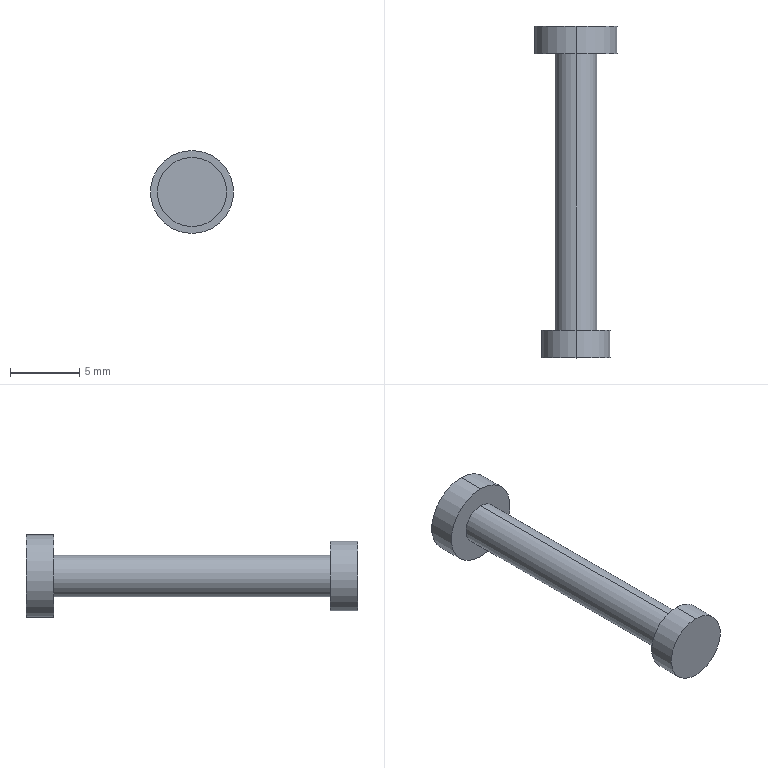Part | SolidWorks | features Revolution 1 | 1 solid | 10 faces | box 6 x 24 x 6 mm | volume 237.19 mm3 | cylinder 6 | plane 4 | commonest cylinder face diameters 3 x2 5 x2 6 x2
STEP:
#1=CARTESIAN_POINT('',(0.,22.,3.));
#2=VERTEX_POINT('',#1);
#3=CARTESIAN_POINT('',(0.,22.,-3.));
#4=VERTEX_POINT('',#3);
#5=CARTESIAN_POINT('',(0.,22.,0.));
#6=DIRECTION('',(0.,1.,0.));
#7=DIRECTION('',(0.,0.,1.));
#8=AXIS2_PLACEMENT_3D('',#5,#6,#7);
#9=CIRCLE('',#8,3.);
#10=EDGE_CURVE('',#2,#4,#9,.T.);
#11=ORIENTED_EDGE('',*,*,#10,.T.);
#12=CARTESIAN_POINT('',(0.,24.,-3.));
#13=VERTEX_POINT('',#12);
#14=CARTESIAN_POINT('',(0.,24.,-3.));
#15=DIRECTION('',(0.,1.,0.));
#16=VECTOR('',#15,1000.);
#17=LINE('',#14,#16);
#18=EDGE_CURVE('',#4,#13,#17,.T.);
#19=ORIENTED_EDGE('',*,*,#18,.T.);
#20=CARTESIAN_POINT('',(0.,24.,3.));
#21=VERTEX_POINT('',#20);
#22=CARTESIAN_POINT('',(0.,24.,0.));
#23=DIRECTION('',(0.,1.,0.));
#24=DIRECTION('',(0.,0.,1.));
#25=AXIS2_PLACEMENT_3D('',#22,#23,#24);
#26=CIRCLE('',#25,3.);
#27=EDGE_CURVE('',#21,#13,#26,.T.);
#28=ORIENTED_EDGE('',*,*,#27,.F.);
#29=CARTESIAN_POINT('',(0.,24.,3.));
#30=DIRECTION('',(0.,1.,0.));
#31=VECTOR('',#30,1000.);
#32=LINE('',#29,#31);
#33=EDGE_CURVE('',#2,#21,#32,.T.);
#34=ORIENTED_EDGE('',*,*,#33,.F.);
#35=EDGE_LOOP('',(#11,#19,#28,#34));
#36=FACE_OUTER_BOUND('',#35,.T.);
#37=CARTESIAN_POINT('',(0.,24.,0.));
#38=DIRECTION('',(0.,1.,0.));
#39=DIRECTION('',(0.,0.,1.));
#40=AXIS2_PLACEMENT_3D('',#37,#38,#39);
#41=CYLINDRICAL_SURFACE('',#40,3.);
#42=ADVANCED_FACE('',(#36),#41,.T.);
#43=CARTESIAN_POINT('',(0.,2.,1.5));
#44=VERTEX_POINT('',#43);
#45=CARTESIAN_POINT('',(0.,2.,-1.5));
#46=VERTEX_POINT('',#45);
#47=CARTESIAN_POINT('',(0.,2.,0.));
#48=DIRECTION('',(0.,1.,0.));
#49=DIRECTION('',(0.,0.,1.));
#50=AXIS2_PLACEMENT_3D('',#47,#48,#49);
#51=CIRCLE('',#50,1.5);
#52=EDGE_CURVE('',#44,#46,#51,.T.);
#53=ORIENTED_EDGE('',*,*,#52,.T.);
#54=CARTESIAN_POINT('',(0.,22.,-1.5));
#55=VERTEX_POINT('',#54);
#56=CARTESIAN_POINT('',(0.,24.,-1.5));
#57=DIRECTION('',(0.,1.,0.));
#58=VECTOR('',#57,1000.);
#59=LINE('',#56,#58);
#60=EDGE_CURVE('',#46,#55,#59,.T.);
#61=ORIENTED_EDGE('',*,*,#60,.T.);
#62=CARTESIAN_POINT('',(0.,22.,1.5));
#63=VERTEX_POINT('',#62);
#64=CARTESIAN_POINT('',(0.,22.,0.));
#65=DIRECTION('',(0.,1.,0.));
#66=DIRECTION('',(0.,0.,1.));
#67=AXIS2_PLACEMENT_3D('',#64,#65,#66);
#68=CIRCLE('',#67,1.5);
#69=EDGE_CURVE('',#63,#55,#68,.T.);
#70=ORIENTED_EDGE('',*,*,#69,.F.);
#71=CARTESIAN_POINT('',(0.,24.,1.5));
#72=DIRECTION('',(0.,1.,0.));
#73=VECTOR('',#72,1000.);
#74=LINE('',#71,#73);
#75=EDGE_CURVE('',#44,#63,#74,.T.);
#76=ORIENTED_EDGE('',*,*,#75,.F.);
#77=EDGE_LOOP('',(#53,#61,#70,#76));
#78=FACE_OUTER_BOUND('',#77,.T.);
#79=CARTESIAN_POINT('',(0.,24.,0.));
#80=DIRECTION('',(0.,1.,0.));
#81=DIRECTION('',(0.,0.,1.));
#82=AXIS2_PLACEMENT_3D('',#79,#80,#81);
#83=CYLINDRICAL_SURFACE('',#82,1.5);
#84=ADVANCED_FACE('',(#78),#83,.T.);
#85=CARTESIAN_POINT('',(0.,0.,2.5));
#86=VERTEX_POINT('',#85);
#87=CARTESIAN_POINT('',(0.,0.,-2.5));
#88=VERTEX_POINT('',#87);
#89=CARTESIAN_POINT('',(0.,0.,0.));
#90=DIRECTION('',(0.,1.,0.));
#91=DIRECTION('',(0.,0.,1.));
#92=AXIS2_PLACEMENT_3D('',#89,#90,#91);
#93=CIRCLE('',#92,2.5);
#94=EDGE_CURVE('',#86,#88,#93,.T.);
#95=ORIENTED_EDGE('',*,*,#94,.T.);
#96=CARTESIAN_POINT('',(0.,2.,-2.5));
#97=VERTEX_POINT('',#96);
#98=CARTESIAN_POINT('',(0.,24.,-2.5));
#99=DIRECTION('',(0.,1.,0.));
#100=VECTOR('',#99,1000.);
#101=LINE('',#98,#100);
#102=EDGE_CURVE('',#88,#97,#101,.T.);
#103=ORIENTED_EDGE('',*,*,#102,.T.);
#104=CARTESIAN_POINT('',(0.,2.,2.5));
#105=VERTEX_POINT('',#104);
#106=CARTESIAN_POINT('',(0.,2.,0.));
#107=DIRECTION('',(0.,1.,0.));
#108=DIRECTION('',(0.,0.,1.));
#109=AXIS2_PLACEMENT_3D('',#106,#107,#108);
#110=CIRCLE('',#109,2.5);
#111=EDGE_CURVE('',#105,#97,#110,.T.);
#112=ORIENTED_EDGE('',*,*,#111,.F.);
#113=CARTESIAN_POINT('',(0.,24.,2.5));
#114=DIRECTION('',(0.,1.,0.));
#115=VECTOR('',#114,1000.);
#116=LINE('',#113,#115);
#117=EDGE_CURVE('',#86,#105,#116,.T.);
#118=ORIENTED_EDGE('',*,*,#117,.F.);
#119=EDGE_LOOP('',(#95,#103,#112,#118));
#120=FACE_OUTER_BOUND('',#119,.T.);
#121=CARTESIAN_POINT('',(0.,24.,0.));
#122=DIRECTION('',(0.,1.,0.));
#123=DIRECTION('',(0.,0.,1.));
#124=AXIS2_PLACEMENT_3D('',#121,#122,#123);
#125=CYLINDRICAL_SURFACE('',#124,2.5);
#126=ADVANCED_FACE('',(#120),#125,.T.);
#127=ORIENTED_EDGE('',*,*,#94,.F.);
#128=CARTESIAN_POINT('',(0.,0.,0.));
#129=DIRECTION('',(0.,1.,0.));
#130=DIRECTION('',(0.,0.,1.));
#131=AXIS2_PLACEMENT_3D('',#128,#129,#130);
#132=CIRCLE('',#131,2.5);
#133=EDGE_CURVE('',#88,#86,#132,.T.);
#134=ORIENTED_EDGE('',*,*,#133,.F.);
#135=EDGE_LOOP('',(#127,#134));
#136=FACE_OUTER_BOUND('',#135,.T.);
#137=CARTESIAN_POINT('',(0.,0.,0.));
#138=DIRECTION('',(0.,1.,0.));
#139=DIRECTION('',(0.,0.,1.));
#140=AXIS2_PLACEMENT_3D('',#137,#138,#139);
#141=PLANE('',#140);
#142=ADVANCED_FACE('',(#136),#141,.F.);
#143=ORIENTED_EDGE('',*,*,#102,.F.);
#144=ORIENTED_EDGE('',*,*,#133,.T.);
#145=ORIENTED_EDGE('',*,*,#117,.T.);
#146=CARTESIAN_POINT('',(0.,2.,0.));
#147=DIRECTION('',(0.,1.,0.));
#148=DIRECTION('',(0.,0.,1.));
#149=AXIS2_PLACEMENT_3D('',#146,#147,#148);
#150=CIRCLE('',#149,2.5);
#151=EDGE_CURVE('',#97,#105,#150,.T.);
#152=ORIENTED_EDGE('',*,*,#151,.F.);
#153=EDGE_LOOP('',(#143,#144,#145,#152));
#154=FACE_OUTER_BOUND('',#153,.T.);
#155=CARTESIAN_POINT('',(0.,24.,0.));
#156=DIRECTION('',(0.,1.,0.));
#157=DIRECTION('',(0.,0.,1.));
#158=AXIS2_PLACEMENT_3D('',#155,#156,#157);
#159=CYLINDRICAL_SURFACE('',#158,2.5);
#160=ADVANCED_FACE('',(#154),#159,.T.);
#161=ORIENTED_EDGE('',*,*,#52,.F.);
#162=CARTESIAN_POINT('',(0.,2.,0.));
#163=DIRECTION('',(0.,1.,0.));
#164=DIRECTION('',(0.,0.,1.));
#165=AXIS2_PLACEMENT_3D('',#162,#163,#164);
#166=CIRCLE('',#165,1.5);
#167=EDGE_CURVE('',#46,#44,#166,.T.);
#168=ORIENTED_EDGE('',*,*,#167,.F.);
#169=EDGE_LOOP('',(#161,#168));
#170=FACE_BOUND('',#169,.T.);
#171=ORIENTED_EDGE('',*,*,#111,.T.);
#172=ORIENTED_EDGE('',*,*,#151,.T.);
#173=EDGE_LOOP('',(#171,#172));
#174=FACE_OUTER_BOUND('',#173,.T.);
#175=CARTESIAN_POINT('',(2.5,2.,0.));
#176=DIRECTION('',(0.,-1.,0.));
#177=DIRECTION('',(0.,0.,-1.));
#178=AXIS2_PLACEMENT_3D('',#175,#176,#177);
#179=PLANE('',#178);
#180=ADVANCED_FACE('',(#170,#174),#179,.F.);
#181=ORIENTED_EDGE('',*,*,#60,.F.);
#182=ORIENTED_EDGE('',*,*,#167,.T.);
#183=ORIENTED_EDGE('',*,*,#75,.T.);
#184=CARTESIAN_POINT('',(0.,22.,0.));
#185=DIRECTION('',(0.,1.,0.));
#186=DIRECTION('',(0.,0.,1.));
#187=AXIS2_PLACEMENT_3D('',#184,#185,#186);
#188=CIRCLE('',#187,1.5);
#189=EDGE_CURVE('',#55,#63,#188,.T.);
#190=ORIENTED_EDGE('',*,*,#189,.F.);
#191=EDGE_LOOP('',(#181,#182,#183,#190));
#192=FACE_OUTER_BOUND('',#191,.T.);
#193=CARTESIAN_POINT('',(0.,24.,0.));
#194=DIRECTION('',(0.,1.,0.));
#195=DIRECTION('',(0.,0.,1.));
#196=AXIS2_PLACEMENT_3D('',#193,#194,#195);
#197=CYLINDRICAL_SURFACE('',#196,1.5);
#198=ADVANCED_FACE('',(#192),#197,.T.);
#199=ORIENTED_EDGE('',*,*,#10,.F.);
#200=CARTESIAN_POINT('',(0.,22.,0.));
#201=DIRECTION('',(0.,1.,0.));
#202=DIRECTION('',(0.,0.,1.));
#203=AXIS2_PLACEMENT_3D('',#200,#201,#202);
#204=CIRCLE('',#203,3.);
#205=EDGE_CURVE('',#4,#2,#204,.T.);
#206=ORIENTED_EDGE('',*,*,#205,.F.);
#207=EDGE_LOOP('',(#199,#206));
#208=FACE_OUTER_BOUND('',#207,.T.);
#209=ORIENTED_EDGE('',*,*,#69,.T.);
#210=ORIENTED_EDGE('',*,*,#189,.T.);
#211=EDGE_LOOP('',(#209,#210));
#212=FACE_BOUND('',#211,.T.);
#213=CARTESIAN_POINT('',(1.5,22.,0.));
#214=DIRECTION('',(0.,1.,0.));
#215=DIRECTION('',(0.,0.,1.));
#216=AXIS2_PLACEMENT_3D('',#213,#214,#215);
#217=PLANE('',#216);
#218=ADVANCED_FACE('',(#208,#212),#217,.F.);
#219=ORIENTED_EDGE('',*,*,#18,.F.);
#220=ORIENTED_EDGE('',*,*,#205,.T.);
#221=ORIENTED_EDGE('',*,*,#33,.T.);
#222=CARTESIAN_POINT('',(0.,24.,0.));
#223=DIRECTION('',(0.,1.,0.));
#224=DIRECTION('',(0.,0.,1.));
#225=AXIS2_PLACEMENT_3D('',#222,#223,#224);
#226=CIRCLE('',#225,3.);
#227=EDGE_CURVE('',#13,#21,#226,.T.);
#228=ORIENTED_EDGE('',*,*,#227,.F.);
#229=EDGE_LOOP('',(#219,#220,#221,#228));
#230=FACE_OUTER_BOUND('',#229,.T.);
#231=CARTESIAN_POINT('',(0.,24.,0.));
#232=DIRECTION('',(0.,1.,0.));
#233=DIRECTION('',(0.,0.,1.));
#234=AXIS2_PLACEMENT_3D('',#231,#232,#233);
#235=CYLINDRICAL_SURFACE('',#234,3.);
#236=ADVANCED_FACE('',(#230),#235,.T.);
#237=ORIENTED_EDGE('',*,*,#27,.T.);
#238=ORIENTED_EDGE('',*,*,#227,.T.);
#239=EDGE_LOOP('',(#237,#238));
#240=FACE_OUTER_BOUND('',#239,.T.);
#241=CARTESIAN_POINT('',(3.,24.,0.));
#242=DIRECTION('',(0.,-1.,0.));
#243=DIRECTION('',(0.,0.,-1.));
#244=AXIS2_PLACEMENT_3D('',#241,#242,#243);
#245=PLANE('',#244);
#246=ADVANCED_FACE('',(#240),#245,.F.);
#247=CLOSED_SHELL('',(#42,#84,#126,#142,#160,#180,#198,#218,#236,#246));
#248=MANIFOLD_SOLID_BREP('',#247);
#249=CARTESIAN_POINT('',(0.,0.,0.));
#250=DIRECTION('',(0.,0.,1.));
#251=DIRECTION('',(1.,0.,0.));
#252=AXIS2_PLACEMENT_3D('',#249,#250,#251);
#253=(LENGTH_UNIT()NAMED_UNIT(*)SI_UNIT(.MILLI.,.METRE.));
#254=UNCERTAINTY_MEASURE_WITH_UNIT(LENGTH_MEASURE(0.00001),#253,'','');
#255=(NAMED_UNIT(*)PLANE_ANGLE_UNIT()SI_UNIT($,.RADIAN.));
#256=(NAMED_UNIT(*)SI_UNIT($,.STERADIAN.)SOLID_ANGLE_UNIT());
#257=(GEOMETRIC_REPRESENTATION_CONTEXT(3)GLOBAL_UNCERTAINTY_ASSIGNED_CONTEXT((#254))GLOBAL_UNIT_ASSIGNED_CONTEXT((#253,#255,#256))REPRESENTATION_CONTEXT('',''));
#258=ADVANCED_BREP_SHAPE_REPRESENTATION('',(#248,#252),#257);